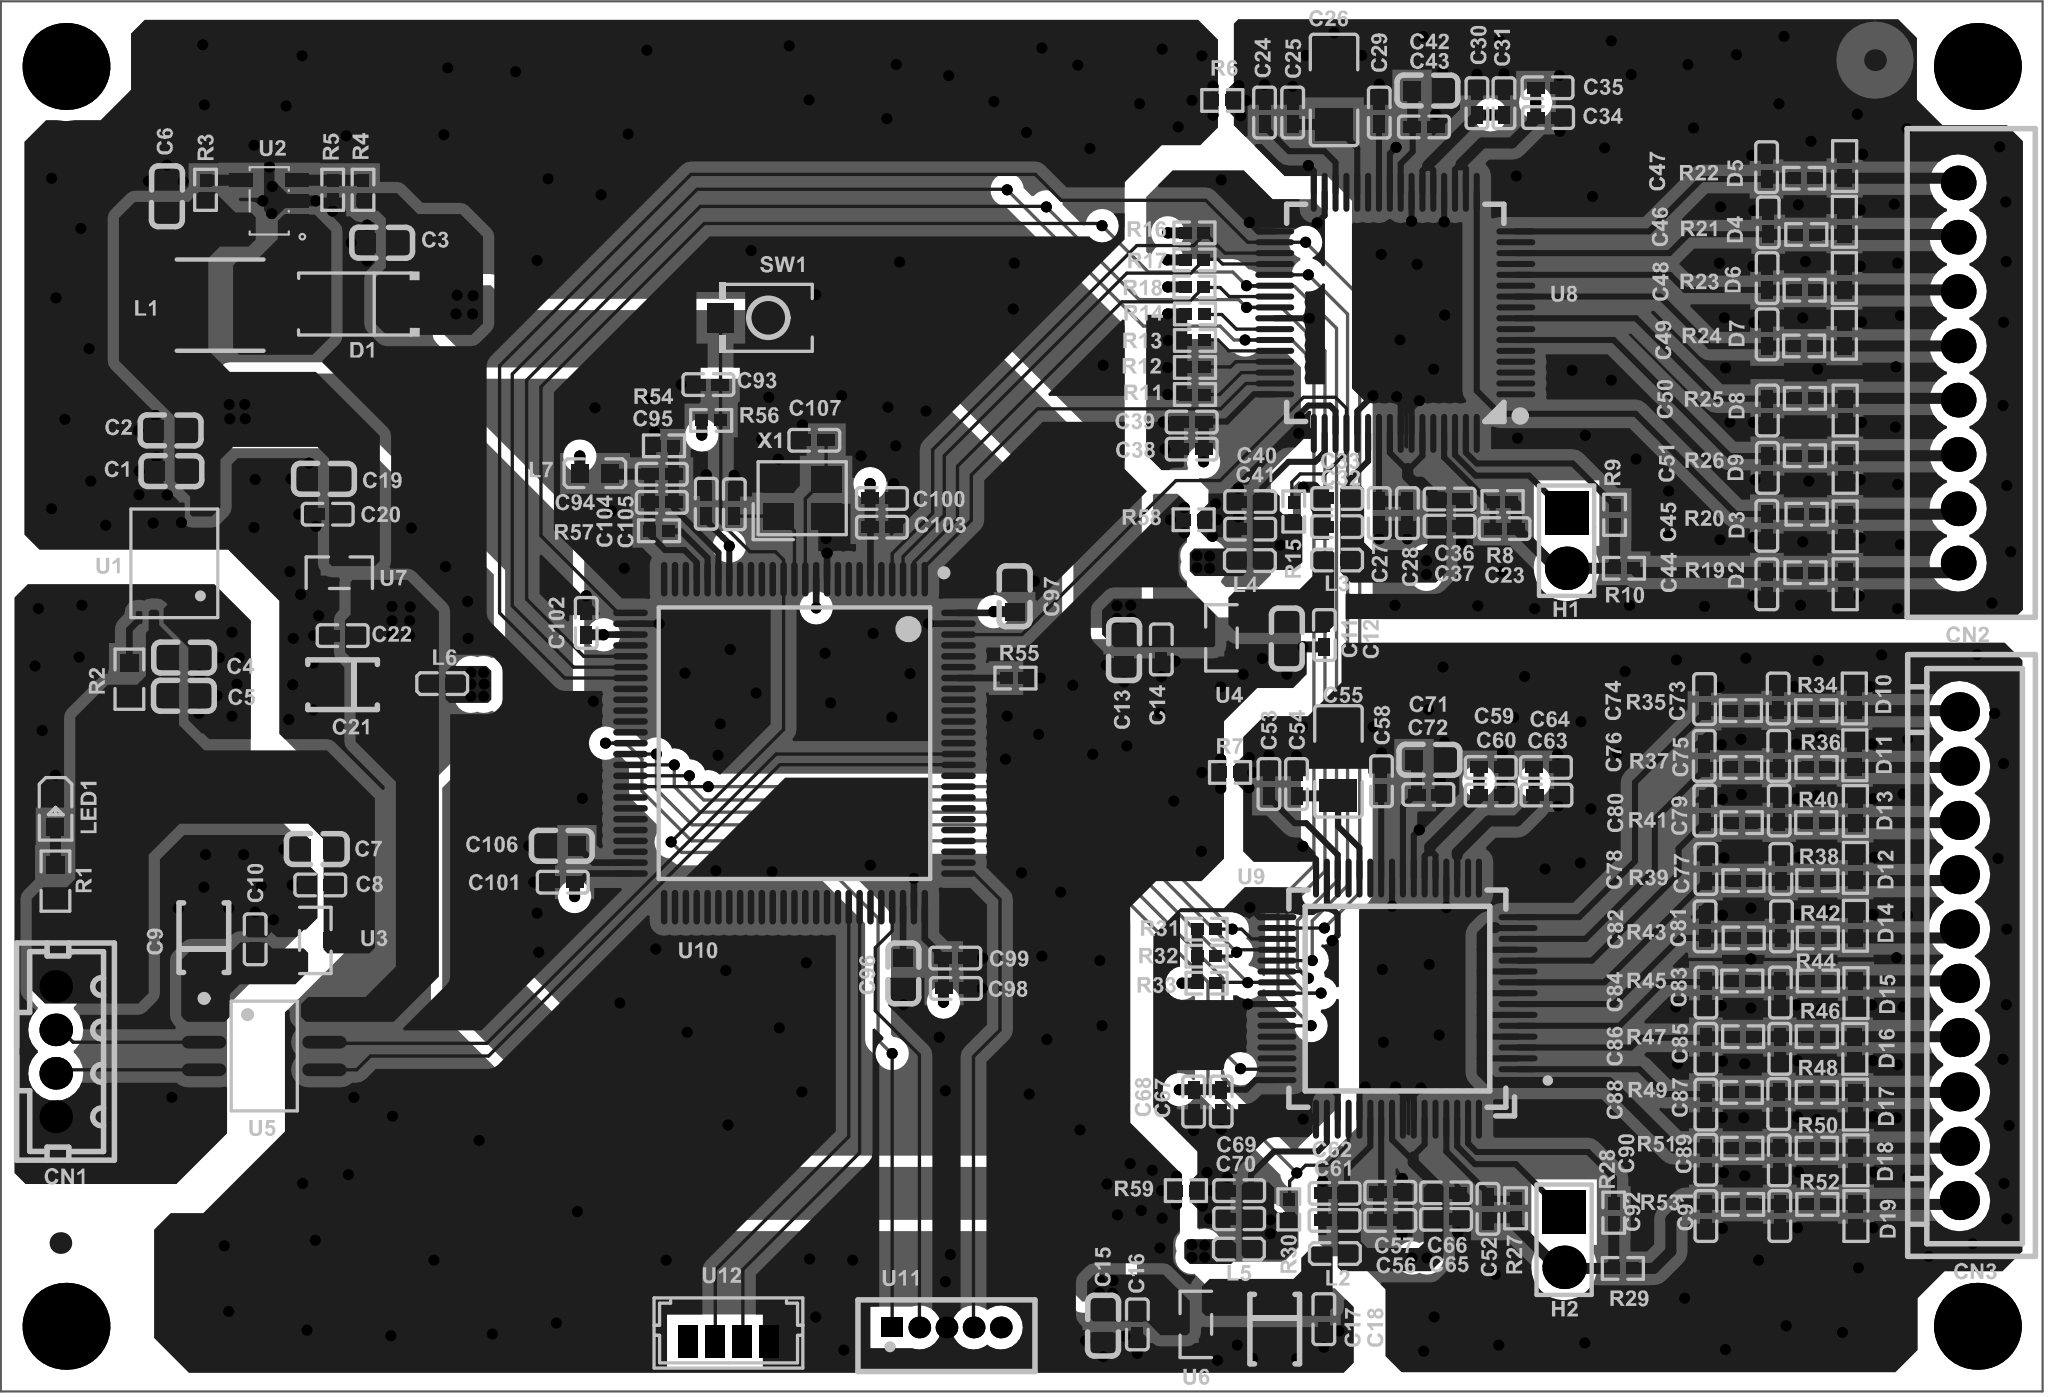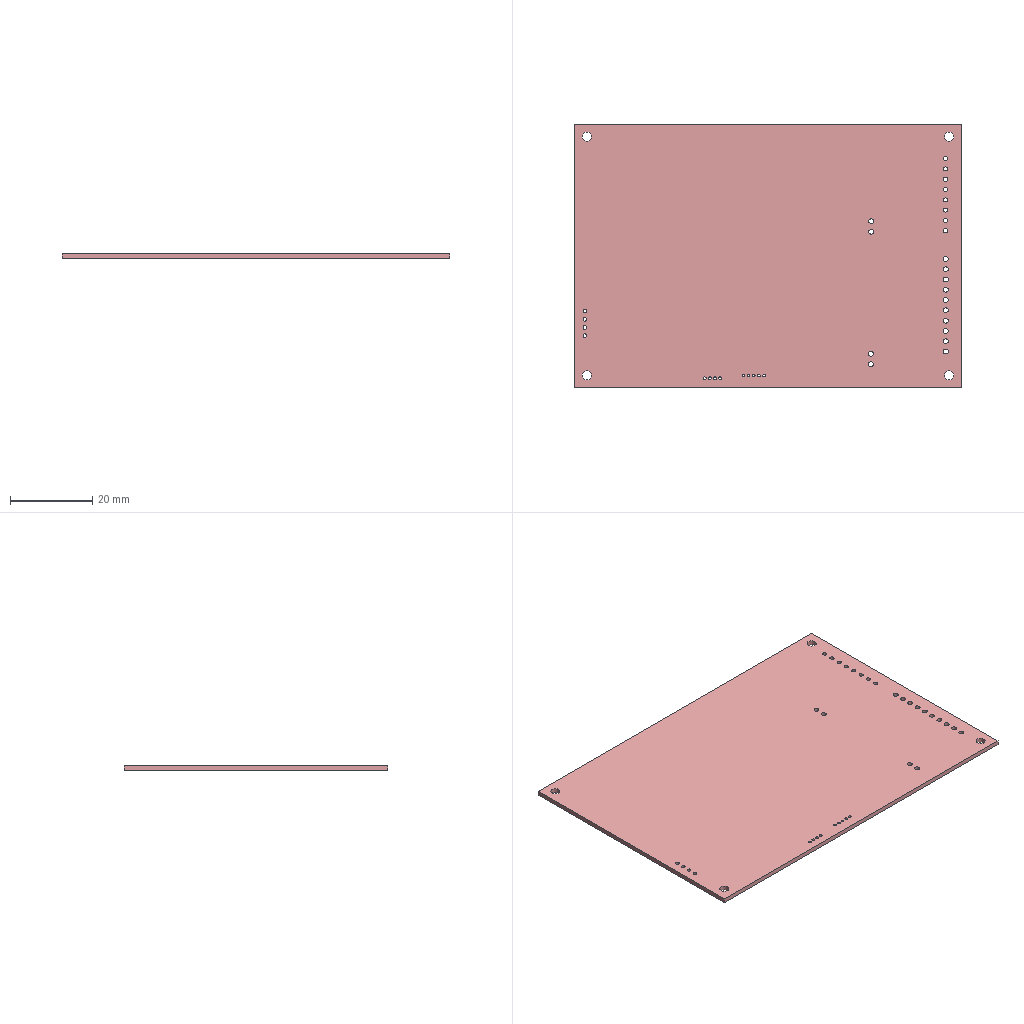Circuit board layout | Altium Designer | box 94 x 64 x 1.1 mm
Part placement:
Designator,Comment,Layer,Footprint,Center-X(mm),Center-Y(mm),Rotation
C1,2.2uF,TopLayer,C0603,7.861,42.367,360
C2,22uF,TopLayer,C0603,7.81,44.247,180
C3,10uF,TopLayer,C0603,17.564,52.883,360
C4,2.2uF,TopLayer,C0603,8.445,33.782,360
C5,22uF,TopLayer,C0603,8.42,32.029,180
C6,10uF,TopLayer,C0603,7.645,55.016,270
C7,10uF,TopLayer,C0603,14.554,24.968,360
C8,1uF,TopLayer,C0402,14.707,23.317,360
C9,22uF,TopLayer,CAP-SMD_L3.2-W1.6,9.347,20.892,90
C10,1uF,TopLayer,C0402,11.709,20.816,270
C11,10uF,TopLayer,C0603,59.207,34.671,90
C12,1uF,TopLayer,C0402,60.935,34.823,90
C13,10uF,TopLayer,C0603,51.714,34.138,90
C14,1uF,TopLayer,C0402,53.427,34.161,90
C15,10uF,TopLayer,C0603,50.749,3.036,90
C16,1uF,TopLayer,C0402,52.324,3.087,90
C17,22uF,TopLayer,CAP-SMD_L3.2-W1.6,58.649,2.87,270
C18,1uF,TopLayer,C0402,60.909,3.327,90
C19,10uF,TopLayer,C0603,14.884,42.012,360
C20,1uF,TopLayer,C0402,15.049,40.386,360
C21,22uF,TopLayer,CAP-SMD_L3.2-W1.6,15.735,32.537,180
C22,1uF,TopLayer,C0402,15.735,34.798,360
C23,10nF,TopLayer,C0402,69.227,39.726,180
C24,1uF,TopLayer,C0402,58.178,58.877,90
C25,1uF,TopLayer,C0402,59.474,58.877,270
C26,100uF,TopLayer,C1206,61.379,59.919,270
C27,1uF,TopLayer,C0402,63.461,40.437,90
C28,100nF,TopLayer,C0402,64.757,40.437,90
C29,1uF,TopLayer,C0402,63.461,58.877,90
C30,1uF,TopLayer,C0402,67.957,59.309,270
C31,100nF,TopLayer,C0402,69.202,59.309,270
C32,1uF,TopLayer,C0402,61.519,39.815,180
C33,100nF,TopLayer,C0402,61.519,41.11,180
C34,1uF,TopLayer,C0402,71.234,58.649,180
C35,100nF,TopLayer,C0402,71.208,60.02,180
C36,1uF,TopLayer,C0402,66.7,41.084,180
C37,100nF,TopLayer,C0402,66.7,39.839,180
C38,1uF,TopLayer,C0402,54.825,43.383,180
C39,100nF,TopLayer,C0402,54.825,44.628,180
C40,1uF,TopLayer,C0402,57.518,40.97,360
C41,100nF,TopLayer,C0402,57.518,39.7,360
C42,10uF,TopLayer,C0603,65.671,59.893,180
C43,100nF,TopLayer,C0402,65.519,58.217,180
C44,4.7nF,TopLayer,C0402,81.304,37.16,90
C45,4.7nF,TopLayer,C0402,81.304,39.853,90
C46,4.7nF,TopLayer,C0402,81.368,53.823,270
C47,4.7nF,TopLayer,C0402,81.292,56.363,270
C48,4.7nF,TopLayer,C0402,81.318,51.257,270
C49,4.7nF,TopLayer,C0402,81.318,48.666,270
C50,4.7nF,TopLayer,C0402,81.33,45.161,90
C51,4.7nF,TopLayer,C0402,81.33,42.52,90
C52,1.5nF,TopLayer,C0402,68.465,8.407,90
C53,1uF,TopLayer,C0402,58.381,27.965,90
C54,1uF,TopLayer,C0402,59.651,27.965,270
C55,22uF,TopLayer,C1206,61.582,29.007,270
C56,1uF,TopLayer,C0402,63.969,7.874,180
C57,100nF,TopLayer,C0402,63.969,9.169,180
C58,1uF,TopLayer,C0402,63.563,28.092,90
C59,1uF,TopLayer,C0402,68.592,28.727,180
C60,100nF,TopLayer,C0402,68.592,27.457,180
C61,1uF,TopLayer,C0402,61.404,7.874,180
C62,100nF,TopLayer,C0402,61.404,9.119,180
C63,1uF,TopLayer,C0402,71.158,27.457,180
C64,100nF,TopLayer,C0402,71.132,28.727,180
C65,1uF,TopLayer,C0402,66.535,7.925,180
C66,100nF,TopLayer,C0402,66.535,9.144,180
C67,1uF,TopLayer,C0402,56.185,13.348,270
C68,100nF,TopLayer,C0402,54.915,13.348,270
C69,1uF,TopLayer,C0402,57.01,9.246,360
C70,100nF,TopLayer,C0402,57.01,7.95,360
C71,10uF,TopLayer,C0603,65.761,29.083,180
C72,100nF,TopLayer,C0402,65.722,27.483,180
C73,47pF,TopLayer,C0402,81.826,31.902,270
C74,47pF,TopLayer,C0402,78.435,31.877,270
C75,47pF,TopLayer,C0402,81.851,29.261,270
C76,47pF,TopLayer,C0402,78.422,29.261,270
C77,47pF,TopLayer,C0402,81.953,24.054,270
C78,47pF,TopLayer,C0402,78.498,24.054,270
C79,47pF,TopLayer,C0402,81.876,26.746,270
C80,47pF,TopLayer,C0402,78.447,26.746,270
C81,47pF,TopLayer,C0402,81.978,21.412,270
C82,47pF,TopLayer,C0402,78.461,21.412,270
C83,47pF,TopLayer,C0402,81.927,18.364,90
C84,47pF,TopLayer,C0402,78.498,18.364,90
C85,47pF,TopLayer,C0402,81.902,15.773,90
C86,47pF,TopLayer,C0402,78.498,15.773,90
C87,47pF,TopLayer,C0402,81.851,13.233,90
C88,47pF,TopLayer,C0402,78.498,13.208,90
C89,47pF,TopLayer,C0402,81.876,10.643,90
C90,47pF,TopLayer,C0402,78.498,10.668,90
C91,47pF,TopLayer,C0402,81.902,8.077,90
C92,47pF,TopLayer,C0402,78.498,8.077,90
C93,100nF,TopLayer,C0402,32.575,46.355,360
C94,100nF,TopLayer,C0402,30.429,40.933,180
C95,1uF,TopLayer,C0402,30.429,42.228,180
C96,2.2uF,TopLayer,C0603,41.554,19.253,90
C97,10uF,TopLayer,C0603,46.672,36.601,270
C98,100nF,TopLayer,C0402,43.967,18.554,180
C99,100nF,TopLayer,C0402,43.942,19.951,180
C100,100nF,TopLayer,C0402,40.564,41.11,180
C101,100nF,TopLayer,C0402,25.869,23.444,360
C102,100nF,TopLayer,C0402,26.949,35.382,270
C103,100nF,TopLayer,C0402,40.564,39.79,180
C104,100nF,TopLayer,C0402,32.473,40.869,270
C105,20pF,TopLayer,C0402,33.769,40.843,270
C106,2.2uF,TopLayer,C0603,25.819,25.121,180
C107,20pF,TopLayer,C0402,37.452,43.79,360
CN1,A2001WV-4P,TopLayer,CONN-TH_A2001WV-4P,2.527,15.646,270
CN2,WF-1A254A8P,TopLayer,CONN-TH_WF-1A254A8P,90.114,46.888,270
CN3,A2501WV-10P,TopLayer,CONN-TH_A2501WV-10P,90.17,20.041,270
D1,B340LA-13-F,TopLayer,SMA_L4.3-W2.6-LS5.2-RD,16.307,50.063,180
D2,TPD1E10B06DPYR-TP,TopLayer,X1-DFN1006-2_L1.0-W0.6-BI,84.911,37.16,90
D3,TPD1E10B06DPYR-TP,TopLayer,X1-DFN1006-2_L1.0-W0.6-BI,84.911,39.827,90
D4,TPD1E10B06DPYR-TP,TopLayer,X1-DFN1006-2_L1.0-W0.6-BI,84.874,53.848,270
D5,TPD1E10B06DPYR-TP,TopLayer,X1-DFN1006-2_L1.0-W0.6-BI,84.887,56.413,270
D6,TPD1E10B06DPYR-TP,TopLayer,X1-DFN1006-2_L1.0-W0.6-BI,84.874,51.257,270
D7,TPD1E10B06DPYR-TP,TopLayer,X1-DFN1006-2_L1.0-W0.6-BI,84.874,48.692,270
D8,TPD1E10B06DPYR-TP,TopLayer,X1-DFN1006-2_L1.0-W0.6-BI,84.911,45.161,90
D9,TPD1E10B06DPYR-TP,TopLayer,X1-DFN1006-2_L1.0-W0.6-BI,84.911,42.52,90
D10,TPD1E10B06DPYR-TP,TopLayer,X1-DFN1006-2_L1.0-W0.6-BI,85.331,31.902,270
D11,TPD1E10B06DPYR-TP,TopLayer,X1-DFN1006-2_L1.0-W0.6-BI,85.356,29.286,270
D12,TPD1E10B06DPYR-TP,TopLayer,X1-DFN1006-2_L1.0-W0.6-BI,85.382,24.105,270
D13,TPD1E10B06DPYR-TP,TopLayer,X1-DFN1006-2_L1.0-W0.6-BI,85.382,26.721,270
D14,TPD1E10B06DPYR-TP,TopLayer,X1-DFN1006-2_L1.0-W0.6-BI,85.382,21.438,270
D15,TPD1E10B06DPYR-TP,TopLayer,X1-DFN1006-2_L1.0-W0.6-BI,85.407,18.339,90
D16,TPD1E10B06DPYR-TP,TopLayer,X1-DFN1006-2_L1.0-W0.6-BI,85.356,15.773,90
D17,TPD1E10B06DPYR-TP,TopLayer,X1-DFN1006-2_L1.0-W0.6-BI,85.382,13.208,90
D18,TPD1E10B06DPYR-TP,TopLayer,X1-DFN1006-2_L1.0-W0.6-BI,85.407,10.643,90
D19,TPD1E10B06DPYR-TP,TopLayer,X1-DFN1006-2_L1.0-W0.6-BI,85.407,8.077,90
H1,PZ254V-11-02P-YL,TopLayer,HDR-TH_2P-P2.54-V-M,72.085,39.167,270
H2,PZ254V-11-02P-YL,TopLayer,HDR-TH_2P-P2.54-V-M,71.97,6.985,270
L1,4.7uH,TopLayer,IND-SMD_L4.0-W4.0_FNR40XXS,10.096,50.013,180
L2,BLM15PD121SN1D,TopLayer,L0402,61.417,6.35,360
L3,BLM15PD121SN1D,TopLayer,L0402,61.519,38.278,360
L4,BLM15PD121SN1D,TopLayer,L0402,57.506,38.252,360
L5,BLM15PD121SN1D,TopLayer,L0402,56.998,6.553,360
L6,BLM15PD121SN1D,TopLayer,L0402,20.32,32.588,360
L7,GZ1608D601TF,TopLayer,L0603,27.356,42.266,360
LED1,KT-0603R,TopLayer,LED0603-RD,2.515,26.772,270
R1,,TopLayer,R0603,2.515,23.495,90
R2,,TopLayer,R0603,5.918,32.791,90
R3,,TopLayer,R0402,9.423,55.321,270
R4,,TopLayer,R0402,16.675,55.321,270
R5,,TopLayer,R0402,15.278,55.321,90
R6,,TopLayer,R0402,56.236,59.436,180
R7,,TopLayer,R0402,56.591,28.499,180
R8,,TopLayer,R0402,69.139,40.97,360
R9,,TopLayer,R0402,74.295,40.361,270
R10,,TopLayer,R0402,74.727,37.897,360
R11,,TopLayer,R0402,54.978,45.898,180
R12,,TopLayer,R0402,54.978,47.142,180
R13,,TopLayer,R0402,54.978,48.387,180
R14,,TopLayer,R0402,54.978,49.606,180
R15,,TopLayer,R0402,59.524,40.513,270
R16,,TopLayer,R0402,54.952,53.34,180
R17,,TopLayer,R0402,54.952,52.095,180
R18,,TopLayer,R0402,54.952,50.851,180
R19,,TopLayer,R0402,83.082,37.694,180
R20,,TopLayer,R0402,83.133,40.386,180
R21,,TopLayer,R0402,83.121,53.264,180
R22,,TopLayer,R0402,83.019,55.855,180
R23,,TopLayer,R0402,83.045,50.698,180
R24,,TopLayer,R0402,83.019,48.133,180
R25,,TopLayer,R0402,83.057,45.72,180
R26,,TopLayer,R0402,83.057,43.078,180
R27,,TopLayer,R0402,69.735,8.433,270
R28,,TopLayer,R0402,74.256,8.23,270
R29,,TopLayer,R0402,74.676,5.664,360
R30,,TopLayer,R0402,59.296,8.382,270
R31,,TopLayer,R0402,55.511,21.285,180
R32,,TopLayer,R0402,55.511,20.041,180
R33,,TopLayer,R0402,55.511,18.796,180
R34,,TopLayer,R0402,83.578,31.344,180
R35,,TopLayer,R0402,80.112,31.344,180
R36,,TopLayer,R0402,83.591,28.727,180
R37,,TopLayer,R0402,80.124,28.727,180
R38,,TopLayer,R0402,83.629,23.52,180
R39,,TopLayer,R0402,80.225,23.52,180
R40,,TopLayer,R0402,83.578,26.187,180
R41,,TopLayer,R0402,80.149,26.187,180
R42,,TopLayer,R0402,83.654,20.879,180
R43,,TopLayer,R0402,80.239,20.879,180
R44,,TopLayer,R0402,83.654,18.898,180
R45,,TopLayer,R0402,80.175,18.898,180
R46,,TopLayer,R0402,83.604,16.332,180
R47,,TopLayer,R0402,80.213,16.332,180
R48,,TopLayer,R0402,83.604,13.767,180
R49,,TopLayer,R0402,80.149,13.767,180
R50,,TopLayer,R0402,83.604,11.201,180
R51,,TopLayer,R0402,80.175,11.201,180
R52,,TopLayer,R0402,83.629,8.611,180
R53,,TopLayer,R0402,80.213,8.611,180
R54,,TopLayer,R0402,30.531,43.536,360
R55,,TopLayer,R0402,46.711,32.842,360
R56,,TopLayer,R0402,32.702,44.704,180
R57,,TopLayer,R0402,30.302,39.624,360
SW1,TS-1088-AR02016,TopLayer,SW-SMD_L3.9-W3.0-P4.45,35.331,49.428,180
U1,,TopLayer,VSON-FCRLF,7.988,38.125,90
U2,MT3540,TopLayer,SOT-23-5_L3.0-W1.7-P0.95-LS2.8-BR,12.357,54.813,360
U3,LN6206P332MR-G,TopLayer,SOT-23-3_L2.9-W1.3-P1.90-LS2.4-BR,14.478,20.765,180
U4,SSP6206-50NR,TopLayer,SOT-23-3_L2.9-W1.3-P1.90-LS2.4-BR,56.195,34.695,360
U5,,TopLayer,SOIC-8_L4.9-W3.9-P1.27-LS6.0-BL,12.128,15.443,270
U6,LN6206P332MR-G,TopLayer,SOT-23-3_L2.9-W1.3-P1.90-LS2.4-BR,55.016,3.087,360
U7,LN6206P332MR-G,TopLayer,SOT-23-3_L2.9-W1.3-P1.90-LS2.4-BR,15.582,37.694,270
U8,ADS1299IPAGR,TopLayer,TQFP-64_L10.0-W10.0-P0.50-LS12.0-TL,64.198,49.657,180
U9,ADS1298IPAGR,TopLayer,TQFP-64_L10.0-W10.0-P0.50-LS12.0-BL,64.3,18.085,90
U10,STM32F407VGT6,TopLayer,LQFP-100_L14.0-W14.0-P0.50-LS16.0-BL,36.537,29.845,180
U11,WAFER-MX1.25-5PZZ,TopLayer,CONN-TH_5P-P1.25_XUNPU_WAFER-MX1.25-5PZZ,43.536,2.946,360
U12,WAFER-MX1.25-4PZZ,TopLayer,CONN-TH_4P-P1.25_WAFER-MX1.25-4PZZ,33.503,2.286,180
X1,8MHz,TopLayer,CRYSTAL-SMD_4P-L3.2-W2.5-BL,36.893,41.123,360
R58,,TopLayer,R0402,54.915,40.132,180
R59,,TopLayer,R0402,54.559,9.246,180